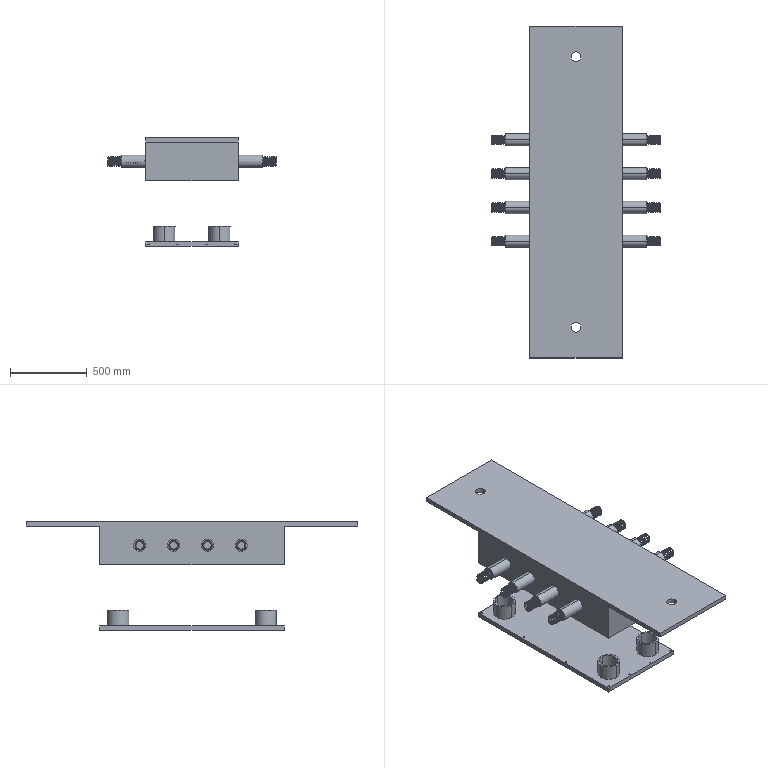Part | SolidWorks | features ReferencePattern 25, LocalLPattern 7, MirrorCompFeat 1, RefAxis 1 | 38 solids | 361 faces | box 1100 x 2160 x 708.763 mm | volume 96729092 mm3 | cylinder 196 | plane 117 | torus 32 | spline 16 | commonest cylinder face diameters 60 x64 10 x48 80 x32 20 x24 120 x16 140 x8